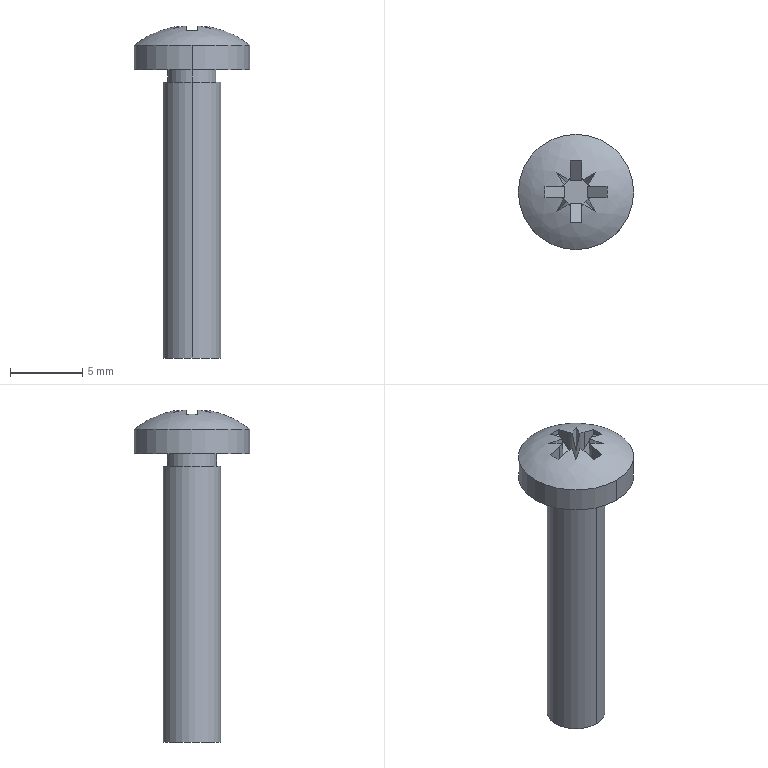Part | SolidWorks | features BaseBody 1 | 1 solid | 51 faces | box 8 x 8 x 23.025 mm | volume 359.622 mm3 | plane 40 | cylinder 10 | spline 1 | commonest cylinder face diameters 1.6 x4 3.4 x2 4 x2 8 x2